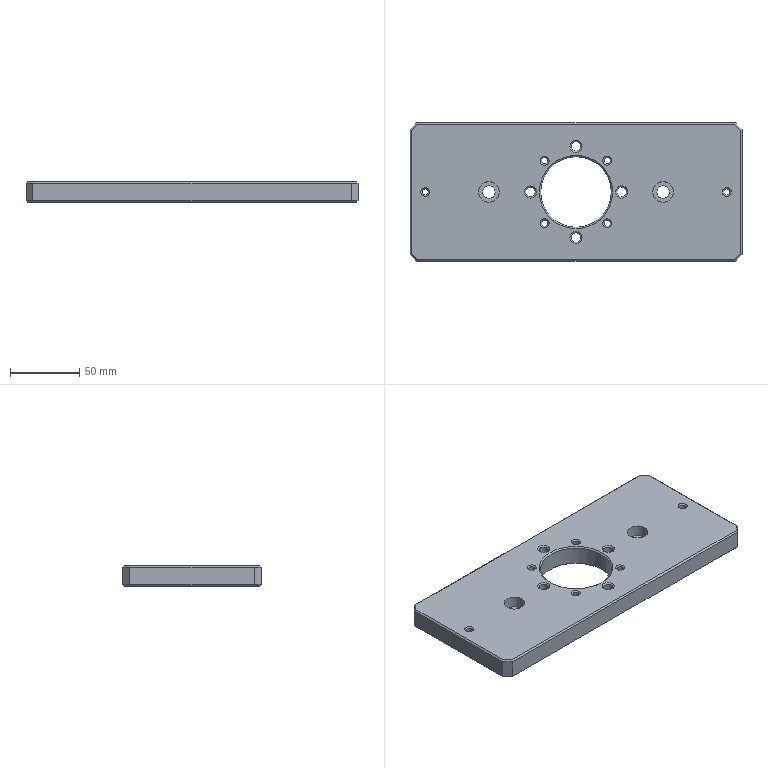Part | STEP file | Wrench mounting plate | 1 solid | 114 faces | box 240 x 100 x 15 mm | volume 319377 mm3 | cone 44 | cylinder 38 | plane 32 | commonest cylinder face diameters 4.5 x12 6.8 x8 8 x8 9 x4 15 x4 51.1 x2